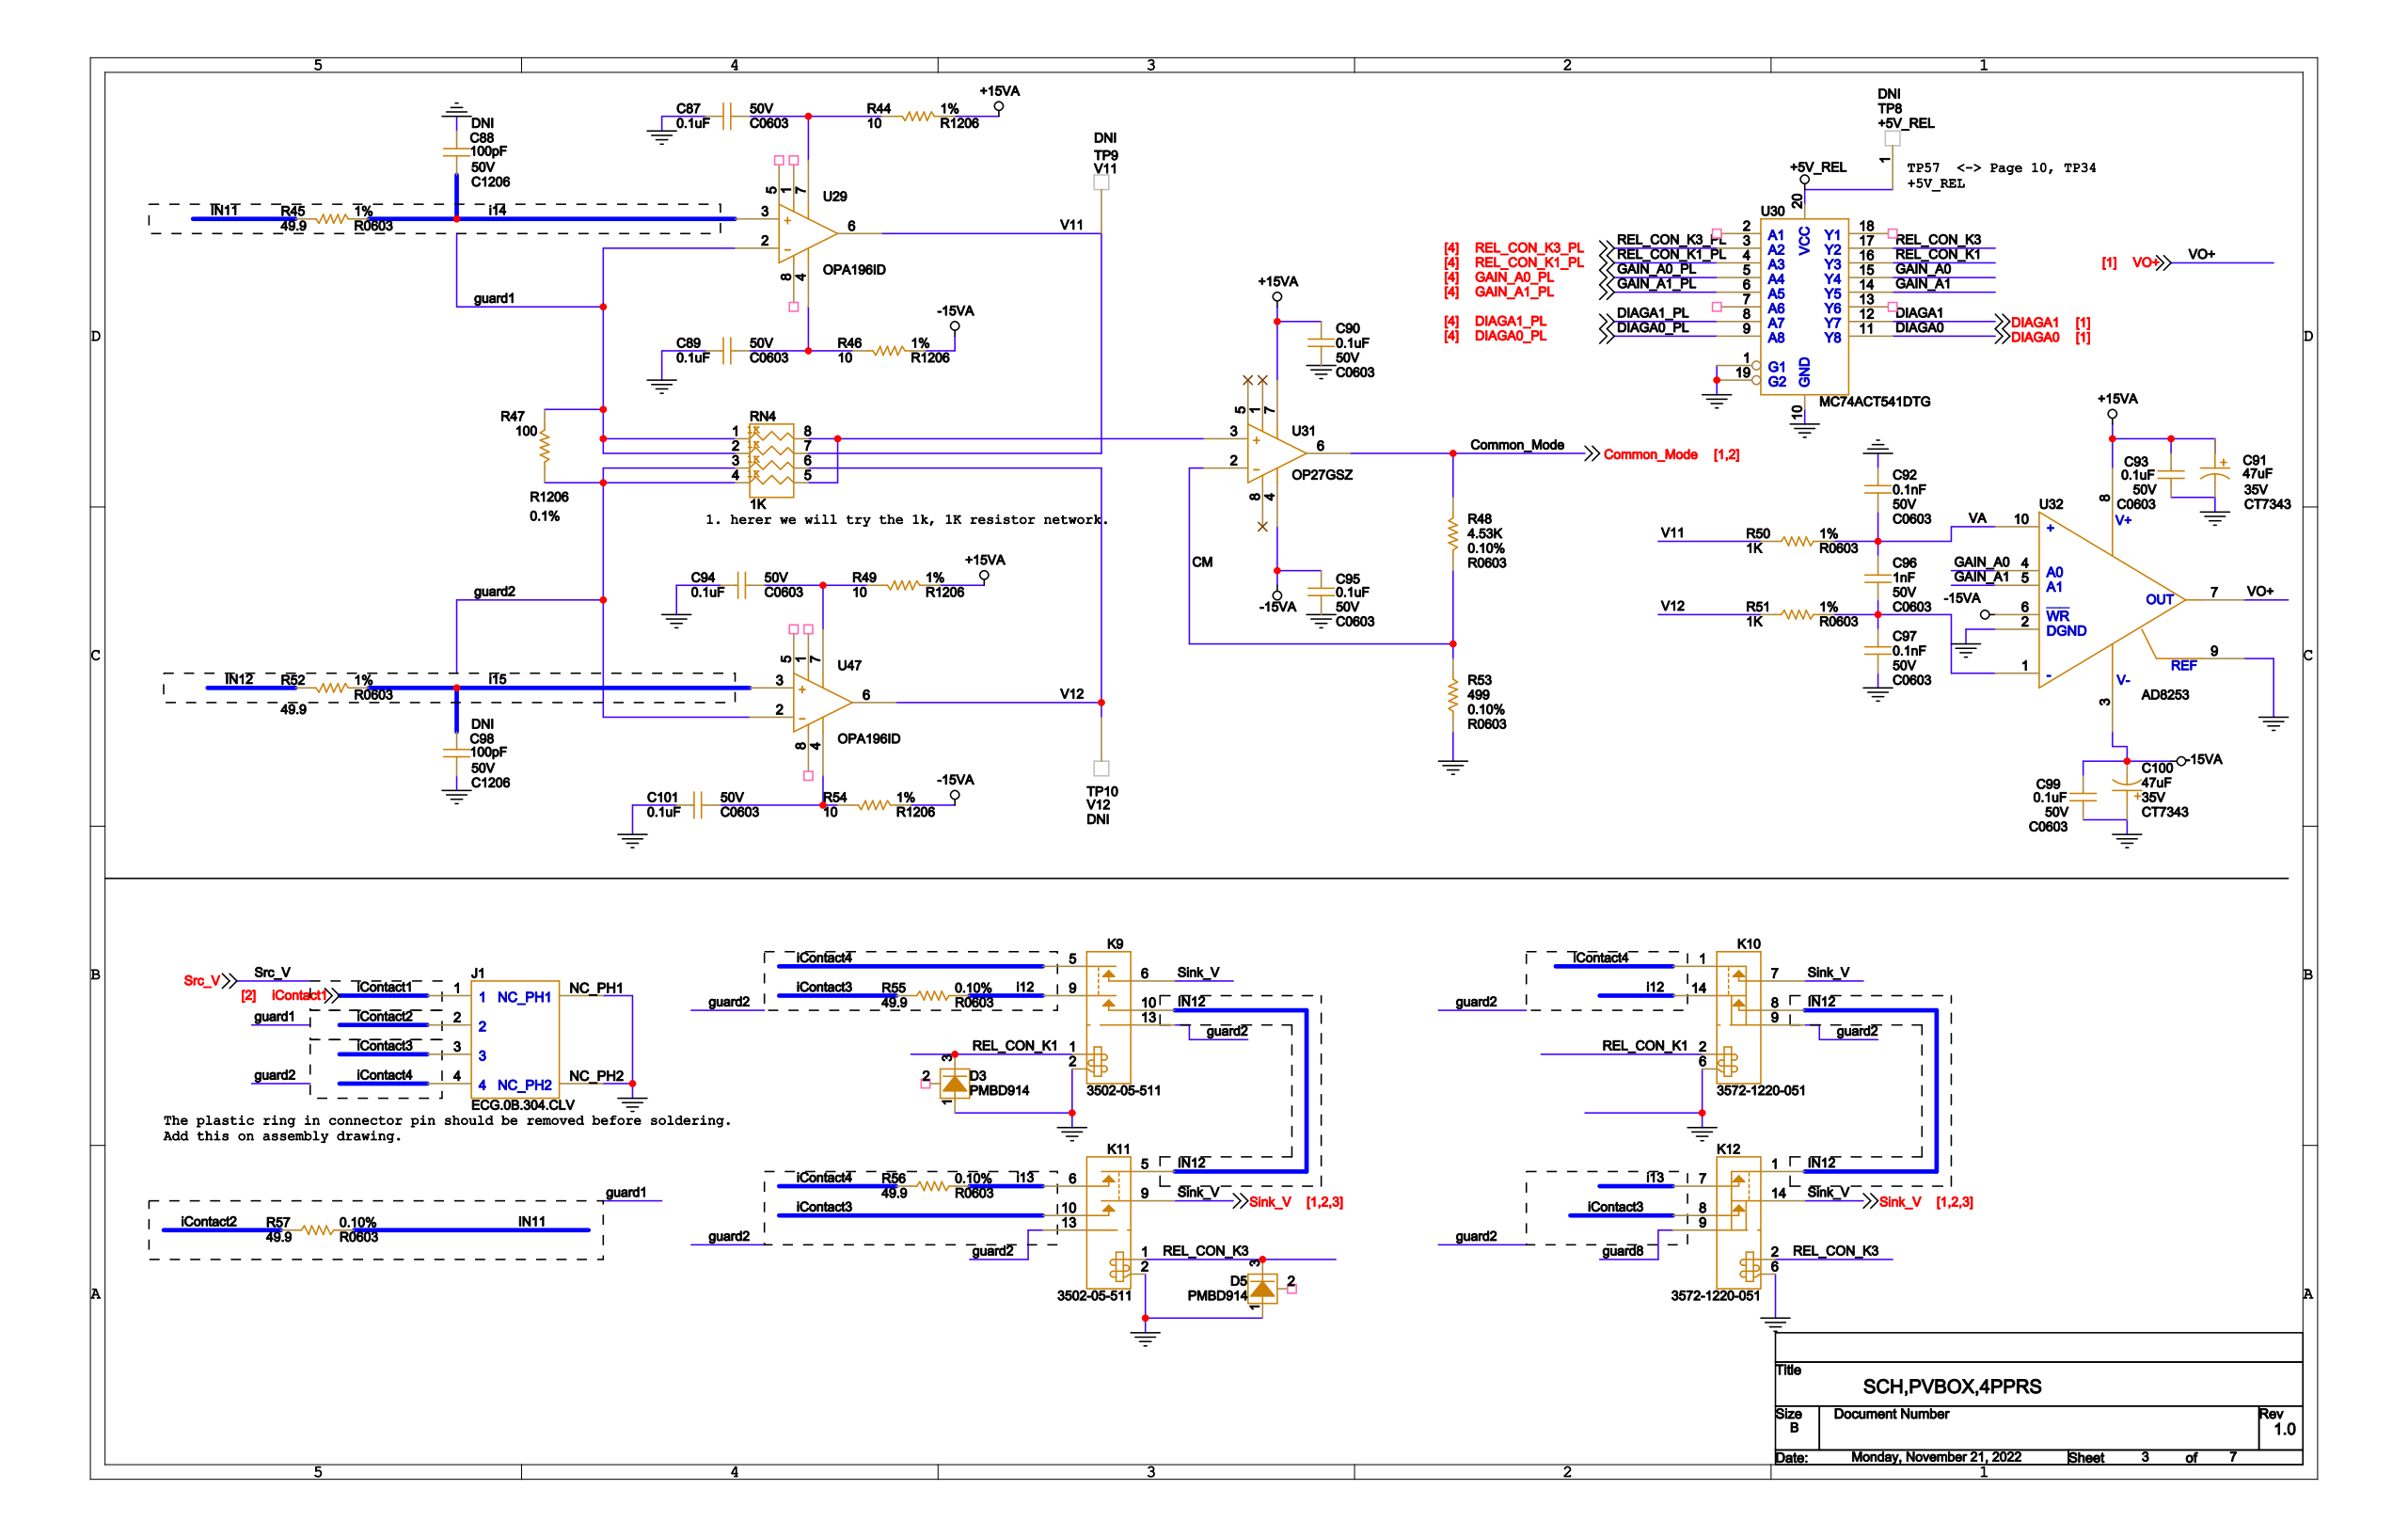Circuit board | Cadence Allegro | 405 parts | 254 nets | one sheet of the schematic
Parts on this sheet (reference | value | footprint):
C87 | C0603
C88 | C1206
C89 | C0603
C90 | C0603
C91 | CT7343
C92 | C0603
C93 | C0603
C94 | C0603
C95 | C0603
C96 | C0603
C97 | C0603
C98 | C1206
C99 | C0603
C100 | CT7343
C101 | C0603
D3 | SOT_3_1M4X3MX1M1_0M95
D5 | SOT_3_1M4X3MX1M1_0M95
K9 | COTO_3502_05_511-A
K10 | COTO_3502_05_511
K11 | COTO_3502_05_511-A
K12 | COTO_3502_05_511
R44 | R1206
R45 | R0603
R46 | R1206
R47 | R1206
R48 | R0603
R49 | R1206
R50 | R0603
R51 | R0603
R52 | R0603
R53 | R0603
R54 | R1206
R55 | R0603
R56 | R0603
R57 | R0603
RN4 | ACASA
TP9 | TP_0M8X1M15
TP10 | TP_0M8X1M15
U29 | SOIC_8_4MX5MX1M75_1M27
U30 | SOPTS_20_4M5X6M6X1M2_0M65
U31 | SOIC_8_4MX5MX1M75_1M27
U32 | SOPM_10_3M1X3M1X1M1_0M5
U47 | SOIC_8_4MX5MX1M75_1M27
Nets of these parts (net: part-pin ...):
GND: C87-1 C88-1 C89-1 C90-2 C91-2 C92-1 C93-2 C94-1 C95-2 C97-2 C98-2 C99-2 C100-1 C101-1 D3-1 D5-1 K9-2 K10-6 K11-2 K12-6 R53-2 U30-1 U30-10 U30-19 U32-2 U32-9
IN11: R45-1 R57-2
I14: C88-2 R45-2 U29-3
IN12: K9-10 K10-8 K11-5 K12-1 R52-1
I15: C98-1 R52-2 U47-3
ICONTACT3: K11-10 K12-8 R55-1
I12: K9-9 K10-14 R55-2
ICONTACT4: K9-5 K10-1 R56-1
I13: K11-6 K12-7 R56-2
ICONTACT2: R57-1
N16799444: C101-2 R54-1 U47-4
+5V_REL: U30-20
+15VA: C90-1 C91-1 C93-1 R44-2 R49-2 U31-7 U32-8
-15VA: C95-1 C99-1 C100-2 R46-2 R54-2 U31-4 U32-3 U32-6
N18629021: C87-2 R44-1 U29-7
N16798939: C89-2 R46-1 U29-4
N16799177: C94-2 R49-1 U47-7
N19318783: C96-1 C97-1 R51-2 U32-1
VA: C92-2 C96-2 R50-2 U32-10
REL_CON_K1: D3-3 K9-1 K10-2 U30-16
REL_CON_K3: D5-3 K11-1 K12-2 U30-17
SINK_V: K9-6 K10-7 K11-9 K12-14
GUARD2: K9-13 K10-9 K11-13 R47-1 RN4-3 RN4-4 U47-2
GUARD8: K12-9
V11: R50-1 RN4-7 TP9-1 U29-6
V12: R51-1 RN4-6 TP10-1 U47-6
COMMON_MODE: R48-2 U31-6
GUARD1: R47-2 RN4-1 RN4-2 U29-2
CM: R48-1 R53-1 U31-2
VO+: U32-7
N17901582: RN4-5 RN4-8 U31-3
REL_CON_K3_PL: U30-3
REL_CON_K1_PL: U30-4
GAIN_A0_PL: U30-5
GAIN_A1_PL: U30-6
DIAGA1_PL: U30-8
DIAGA0_PL: U30-9
GAIN_A0: U30-15 U32-4
GAIN_A1: U30-14 U32-5
DIAGA1: U30-12
DIAGA0: U30-11